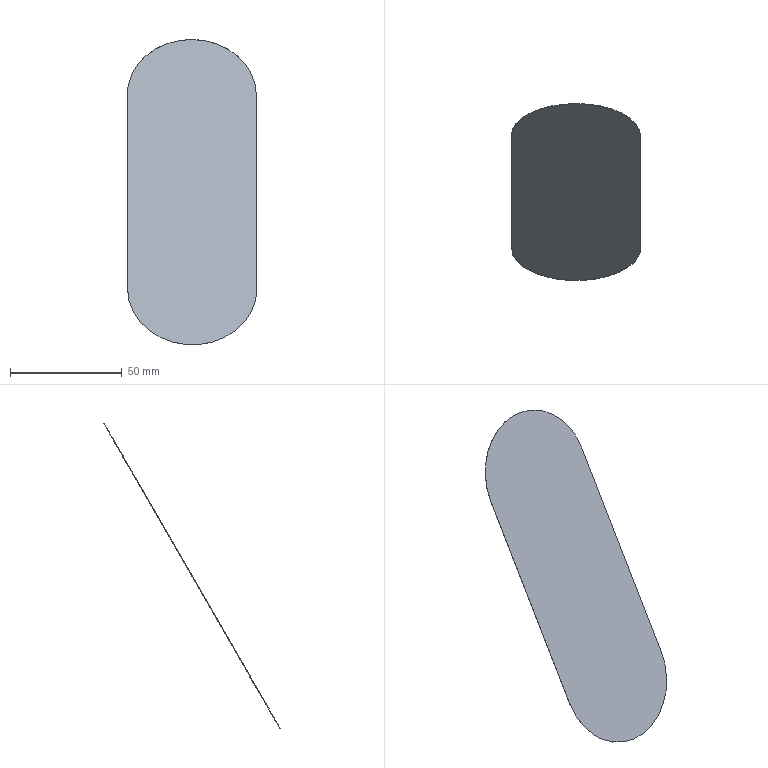Part | SolidWorks | features BaseBody 1 | 1 solid | 7 faces | box 58.218 x 79.087 x 136.882 mm | volume 844.208 mm3 | plane 4 | cylinder 3 | commonest cylinder face diameters 58 x3
STEP:
#1=CARTESIAN_POINT('',(742.93,77.295,107.762));
#2=VERTEX_POINT('',#1);
#3=CARTESIAN_POINT('',(713.93,62.668,82.647));
#4=VERTEX_POINT('',#3);
#5=CARTESIAN_POINT('',(742.93,62.795,82.647));
#6=DIRECTION('',(0.003769,-0.866,0.5));
#7=DIRECTION('',(0.,0.5,0.866));
#8=AXIS2_PLACEMENT_3D('',#5,#6,#7);
#9=CIRCLE('',#8,29.);
#10=EDGE_CURVE('',#2,#4,#9,.T.);
#11=ORIENTED_EDGE('',*,*,#10,.F.);
#12=CARTESIAN_POINT('',(742.93,77.381,107.712));
#13=VERTEX_POINT('',#12);
#14=CARTESIAN_POINT('',(742.93,77.381,107.712));
#15=DIRECTION('',(-0.003769,0.866,-0.5));
#16=VECTOR('',#15,1000.);
#17=LINE('',#14,#16);
#18=EDGE_CURVE('',#2,#13,#17,.T.);
#19=ORIENTED_EDGE('',*,*,#18,.T.);
#20=CARTESIAN_POINT('',(713.93,62.755,82.597));
#21=VERTEX_POINT('',#20);
#22=CARTESIAN_POINT('',(742.93,62.881,82.597));
#23=DIRECTION('',(0.003769,-0.866,0.5));
#24=DIRECTION('',(0.,0.5,0.866));
#25=AXIS2_PLACEMENT_3D('',#22,#23,#24);
#26=CIRCLE('',#25,29.);
#27=EDGE_CURVE('',#13,#21,#26,.T.);
#28=ORIENTED_EDGE('',*,*,#27,.T.);
#29=CARTESIAN_POINT('',(713.93,62.755,82.597));
#30=DIRECTION('',(0.003769,-0.866,0.5));
#31=VECTOR('',#30,1000.);
#32=LINE('',#29,#31);
#33=EDGE_CURVE('',#21,#4,#32,.T.);
#34=ORIENTED_EDGE('',*,*,#33,.T.);
#35=EDGE_LOOP('',(#11,#19,#28,#34));
#36=FACE_OUTER_BOUND('',#35,.T.);
#37=CARTESIAN_POINT('',(742.93,62.881,82.597));
#38=DIRECTION('',(-0.003769,0.866,-0.5));
#39=DIRECTION('',(0.,0.5,0.866));
#40=AXIS2_PLACEMENT_3D('',#37,#38,#39);
#41=CYLINDRICAL_SURFACE('',#40,29.);
#42=ADVANCED_FACE('',(#36),#41,.T.);
#43=CARTESIAN_POINT('',(714.148,12.669,-3.955));
#44=VERTEX_POINT('',#43);
#45=CARTESIAN_POINT('',(713.93,62.668,82.647));
#46=DIRECTION('',(0.002176,-0.5,-0.866));
#47=VECTOR('',#46,1000.);
#48=LINE('',#45,#47);
#49=EDGE_CURVE('',#4,#44,#48,.T.);
#50=ORIENTED_EDGE('',*,*,#49,.T.);
#51=CARTESIAN_POINT('',(772.148,12.921,-3.955));
#52=VERTEX_POINT('',#51);
#53=CARTESIAN_POINT('',(743.148,12.795,-3.955));
#54=DIRECTION('',(0.003769,-0.866,0.5));
#55=DIRECTION('',(0.,0.5,0.866));
#56=AXIS2_PLACEMENT_3D('',#53,#54,#55);
#57=CIRCLE('',#56,29.);
#58=EDGE_CURVE('',#44,#52,#57,.T.);
#59=ORIENTED_EDGE('',*,*,#58,.T.);
#60=CARTESIAN_POINT('',(771.93,62.921,82.647));
#61=VERTEX_POINT('',#60);
#62=CARTESIAN_POINT('',(772.148,12.921,-3.955));
#63=DIRECTION('',(-0.002176,0.5,0.866));
#64=VECTOR('',#63,1000.);
#65=LINE('',#62,#64);
#66=EDGE_CURVE('',#52,#61,#65,.T.);
#67=ORIENTED_EDGE('',*,*,#66,.T.);
#68=CARTESIAN_POINT('',(742.93,62.795,82.647));
#69=DIRECTION('',(0.003769,-0.866,0.5));
#70=DIRECTION('',(0.,0.5,0.866));
#71=AXIS2_PLACEMENT_3D('',#68,#69,#70);
#72=CIRCLE('',#71,29.);
#73=EDGE_CURVE('',#61,#2,#72,.T.);
#74=ORIENTED_EDGE('',*,*,#73,.T.);
#75=ORIENTED_EDGE('',*,*,#10,.T.);
#76=EDGE_LOOP('',(#50,#59,#67,#74,#75));
#77=FACE_OUTER_BOUND('',#76,.T.);
#78=CARTESIAN_POINT('',(743.039,37.795,39.346));
#79=DIRECTION('',(0.003769,-0.866,0.5));
#80=DIRECTION('',(0.,-0.5,-0.866));
#81=AXIS2_PLACEMENT_3D('',#78,#79,#80);
#82=PLANE('',#81);
#83=ADVANCED_FACE('',(#77),#82,.T.);
#84=CARTESIAN_POINT('',(714.148,12.755,-4.005));
#85=VERTEX_POINT('',#84);
#86=CARTESIAN_POINT('',(714.148,12.755,-4.005));
#87=DIRECTION('',(-0.003769,0.866,-0.5));
#88=VECTOR('',#87,1000.);
#89=LINE('',#86,#88);
#90=EDGE_CURVE('',#44,#85,#89,.T.);
#91=ORIENTED_EDGE('',*,*,#90,.T.);
#92=CARTESIAN_POINT('',(772.147,13.008,-4.005));
#93=VERTEX_POINT('',#92);
#94=CARTESIAN_POINT('',(743.147,12.882,-4.005));
#95=DIRECTION('',(0.003769,-0.866,0.5));
#96=DIRECTION('',(0.,0.5,0.866));
#97=AXIS2_PLACEMENT_3D('',#94,#95,#96);
#98=CIRCLE('',#97,29.);
#99=EDGE_CURVE('',#85,#93,#98,.T.);
#100=ORIENTED_EDGE('',*,*,#99,.T.);
#101=CARTESIAN_POINT('',(772.147,13.008,-4.005));
#102=DIRECTION('',(0.003769,-0.866,0.5));
#103=VECTOR('',#102,1000.);
#104=LINE('',#101,#103);
#105=EDGE_CURVE('',#93,#52,#104,.T.);
#106=ORIENTED_EDGE('',*,*,#105,.T.);
#107=ORIENTED_EDGE('',*,*,#58,.F.);
#108=EDGE_LOOP('',(#91,#100,#106,#107));
#109=FACE_OUTER_BOUND('',#108,.T.);
#110=CARTESIAN_POINT('',(743.147,12.882,-4.005));
#111=DIRECTION('',(-0.003769,0.866,-0.5));
#112=DIRECTION('',(0.,0.5,0.866));
#113=AXIS2_PLACEMENT_3D('',#110,#111,#112);
#114=CYLINDRICAL_SURFACE('',#113,29.);
#115=ADVANCED_FACE('',(#109),#114,.T.);
#116=ORIENTED_EDGE('',*,*,#90,.F.);
#117=ORIENTED_EDGE('',*,*,#49,.F.);
#118=ORIENTED_EDGE('',*,*,#33,.F.);
#119=CARTESIAN_POINT('',(714.148,12.755,-4.005));
#120=DIRECTION('',(-0.002176,0.5,0.866));
#121=VECTOR('',#120,1000.);
#122=LINE('',#119,#121);
#123=EDGE_CURVE('',#85,#21,#122,.T.);
#124=ORIENTED_EDGE('',*,*,#123,.F.);
#125=EDGE_LOOP('',(#116,#117,#118,#124));
#126=FACE_OUTER_BOUND('',#125,.T.);
#127=CARTESIAN_POINT('',(714.039,37.755,39.296));
#128=DIRECTION('',(1.,0.004352,-0.000000001));
#129=DIRECTION('',(-0.004352,1.,0.));
#130=AXIS2_PLACEMENT_3D('',#127,#128,#129);
#131=PLANE('',#130);
#132=ADVANCED_FACE('',(#126),#131,.F.);
#133=ORIENTED_EDGE('',*,*,#18,.F.);
#134=ORIENTED_EDGE('',*,*,#73,.F.);
#135=CARTESIAN_POINT('',(771.93,63.007,82.597));
#136=VERTEX_POINT('',#135);
#137=CARTESIAN_POINT('',(771.93,63.007,82.597));
#138=DIRECTION('',(-0.003769,0.866,-0.5));
#139=VECTOR('',#138,1000.);
#140=LINE('',#137,#139);
#141=EDGE_CURVE('',#61,#136,#140,.T.);
#142=ORIENTED_EDGE('',*,*,#141,.T.);
#143=CARTESIAN_POINT('',(742.93,62.881,82.597));
#144=DIRECTION('',(0.003769,-0.866,0.5));
#145=DIRECTION('',(0.,0.5,0.866));
#146=AXIS2_PLACEMENT_3D('',#143,#144,#145);
#147=CIRCLE('',#146,29.);
#148=EDGE_CURVE('',#136,#13,#147,.T.);
#149=ORIENTED_EDGE('',*,*,#148,.T.);
#150=EDGE_LOOP('',(#133,#134,#142,#149));
#151=FACE_OUTER_BOUND('',#150,.T.);
#152=CARTESIAN_POINT('',(742.93,62.881,82.597));
#153=DIRECTION('',(-0.003769,0.866,-0.5));
#154=DIRECTION('',(0.,0.5,0.866));
#155=AXIS2_PLACEMENT_3D('',#152,#153,#154);
#156=CYLINDRICAL_SURFACE('',#155,29.);
#157=ADVANCED_FACE('',(#151),#156,.T.);
#158=ORIENTED_EDGE('',*,*,#141,.F.);
#159=ORIENTED_EDGE('',*,*,#66,.F.);
#160=ORIENTED_EDGE('',*,*,#105,.F.);
#161=CARTESIAN_POINT('',(771.93,63.007,82.597));
#162=DIRECTION('',(0.002176,-0.5,-0.866));
#163=VECTOR('',#162,1000.);
#164=LINE('',#161,#163);
#165=EDGE_CURVE('',#136,#93,#164,.T.);
#166=ORIENTED_EDGE('',*,*,#165,.F.);
#167=EDGE_LOOP('',(#158,#159,#160,#166));
#168=FACE_OUTER_BOUND('',#167,.T.);
#169=CARTESIAN_POINT('',(772.038,38.008,39.296));
#170=DIRECTION('',(-1.,-0.004352,0.000000001));
#171=DIRECTION('',(0.004352,-1.,0.));
#172=AXIS2_PLACEMENT_3D('',#169,#170,#171);
#173=PLANE('',#172);
#174=ADVANCED_FACE('',(#168),#173,.F.);
#175=ORIENTED_EDGE('',*,*,#99,.F.);
#176=ORIENTED_EDGE('',*,*,#123,.T.);
#177=ORIENTED_EDGE('',*,*,#27,.F.);
#178=ORIENTED_EDGE('',*,*,#148,.F.);
#179=ORIENTED_EDGE('',*,*,#165,.T.);
#180=EDGE_LOOP('',(#175,#176,#177,#178,#179));
#181=FACE_OUTER_BOUND('',#180,.T.);
#182=CARTESIAN_POINT('',(743.039,37.881,39.296));
#183=DIRECTION('',(0.003769,-0.866,0.5));
#184=DIRECTION('',(0.,-0.5,-0.866));
#185=AXIS2_PLACEMENT_3D('',#182,#183,#184);
#186=PLANE('',#185);
#187=ADVANCED_FACE('',(#181),#186,.F.);
#188=CLOSED_SHELL('',(#42,#83,#115,#132,#157,#174,#187));
#189=MANIFOLD_SOLID_BREP('',#188);
#190=CARTESIAN_POINT('',(0.,0.,0.));
#191=DIRECTION('',(0.,0.,1.));
#192=DIRECTION('',(1.,0.,0.));
#193=AXIS2_PLACEMENT_3D('',#190,#191,#192);
#194=(LENGTH_UNIT()NAMED_UNIT(*)SI_UNIT(.MILLI.,.METRE.));
#195=UNCERTAINTY_MEASURE_WITH_UNIT(LENGTH_MEASURE(0.00001),#194,'','');
#196=(NAMED_UNIT(*)PLANE_ANGLE_UNIT()SI_UNIT($,.RADIAN.));
#197=(NAMED_UNIT(*)SI_UNIT($,.STERADIAN.)SOLID_ANGLE_UNIT());
#198=(GEOMETRIC_REPRESENTATION_CONTEXT(3)GLOBAL_UNCERTAINTY_ASSIGNED_CONTEXT((#195))GLOBAL_UNIT_ASSIGNED_CONTEXT((#194,#196,#197))REPRESENTATION_CONTEXT('',''));
#199=ADVANCED_BREP_SHAPE_REPRESENTATION('',(#189,#193),#198);